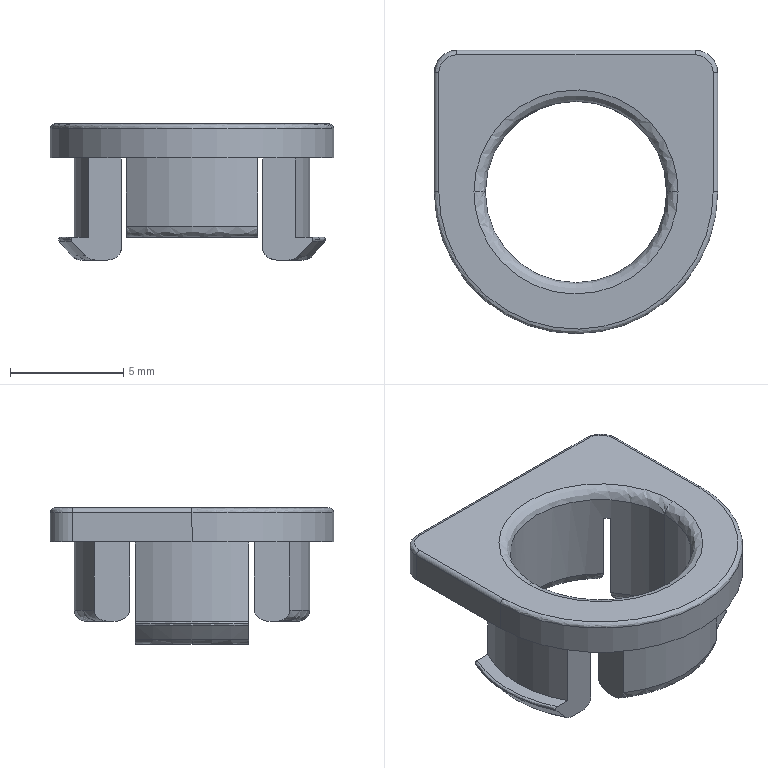Part | SolidWorks | features BaseBody 1 | 1 solid | 55 faces | box 12.5 x 12.5 x 6 mm | volume 243.257 mm3 | spline 20 | plane 19 | cylinder 13 | cone 3 | commonest cylinder face diameters 10.4 x5 0.4 x3 2 x2 8 x2 12.5 x1